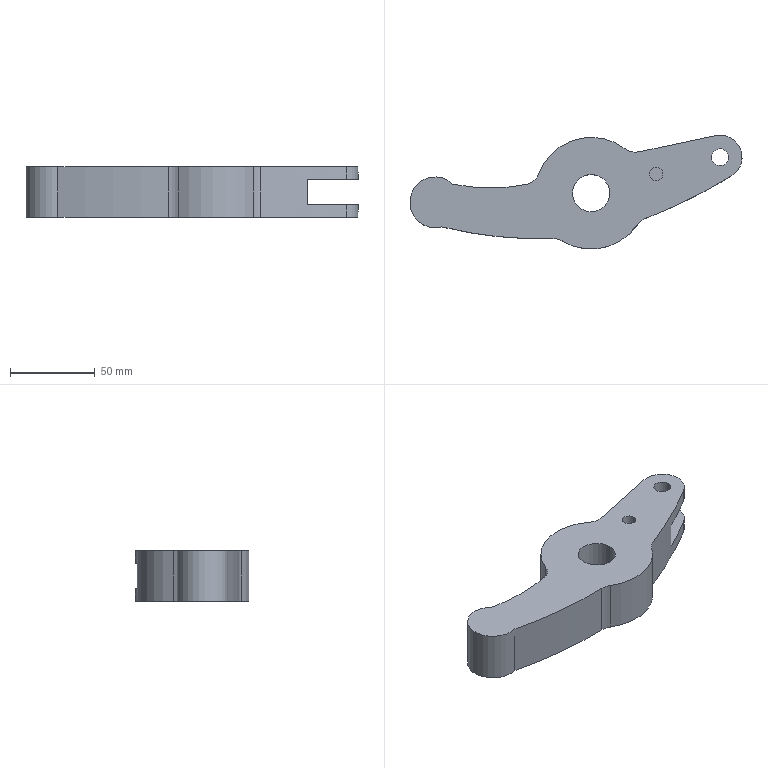Part | SolidWorks | features ICE 15, Cut 1, Extrusion 1, Fillet 1 | 1 solid | 27 faces | box 196.199 x 67.267 x 30 mm | volume 199091 mm3 | cylinder 20 | plane 7 | commonest cylinder face diameters 10 x4 20 x4 8 x2 22 x2 26 x2 66 x2
STEP:
#1=CARTESIAN_POINT('',(135.128,11.377,5.));
#2=VERTEX_POINT('',#1);
#3=CARTESIAN_POINT('',(143.128,11.377,5.));
#4=VERTEX_POINT('',#3);
#5=CARTESIAN_POINT('',(139.128,11.377,5.));
#6=DIRECTION('',(0.,0.,1.));
#7=DIRECTION('',(1.,0.,0.));
#8=AXIS2_PLACEMENT_3D('',#5,#6,#7);
#9=CIRCLE('',#8,4.);
#10=EDGE_CURVE('',#2,#4,#9,.T.);
#11=ORIENTED_EDGE('',*,*,#10,.F.);
#12=CARTESIAN_POINT('',(135.128,11.377,20.));
#13=VERTEX_POINT('',#12);
#14=CARTESIAN_POINT('',(135.128,11.377,5.));
#15=DIRECTION('',(0.,0.,1.));
#16=VECTOR('',#15,1000.);
#17=LINE('',#14,#16);
#18=EDGE_CURVE('',#2,#13,#17,.T.);
#19=ORIENTED_EDGE('',*,*,#18,.T.);
#20=CARTESIAN_POINT('',(143.128,11.377,20.));
#21=VERTEX_POINT('',#20);
#22=CARTESIAN_POINT('',(139.128,11.377,20.));
#23=DIRECTION('',(0.,0.,1.));
#24=DIRECTION('',(1.,0.,0.));
#25=AXIS2_PLACEMENT_3D('',#22,#23,#24);
#26=CIRCLE('',#25,4.);
#27=EDGE_CURVE('',#13,#21,#26,.T.);
#28=ORIENTED_EDGE('',*,*,#27,.T.);
#29=CARTESIAN_POINT('',(143.128,11.377,5.));
#30=DIRECTION('',(0.,0.,1.));
#31=VECTOR('',#30,1000.);
#32=LINE('',#29,#31);
#33=EDGE_CURVE('',#4,#21,#32,.T.);
#34=ORIENTED_EDGE('',*,*,#33,.F.);
#35=EDGE_LOOP('',(#11,#19,#28,#34));
#36=FACE_OUTER_BOUND('',#35,.T.);
#37=CARTESIAN_POINT('',(139.128,11.377,5.));
#38=DIRECTION('',(0.,0.,1.));
#39=DIRECTION('',(1.,0.,0.));
#40=AXIS2_PLACEMENT_3D('',#37,#38,#39);
#41=CYLINDRICAL_SURFACE('',#40,4.);
#42=ADVANCED_FACE('',(#36),#41,.F.);
#43=CARTESIAN_POINT('',(111.78,0.,20.));
#44=VERTEX_POINT('',#43);
#45=CARTESIAN_POINT('',(89.78,0.,20.));
#46=VERTEX_POINT('',#45);
#47=CARTESIAN_POINT('',(100.78,0.,20.));
#48=DIRECTION('',(0.,0.,-1.));
#49=DIRECTION('',(-1.,0.,0.));
#50=AXIS2_PLACEMENT_3D('',#47,#48,#49);
#51=CIRCLE('',#50,11.);
#52=EDGE_CURVE('',#44,#46,#51,.T.);
#53=ORIENTED_EDGE('',*,*,#52,.F.);
#54=CARTESIAN_POINT('',(111.78,0.,-10.));
#55=VERTEX_POINT('',#54);
#56=CARTESIAN_POINT('',(111.78,0.,20.));
#57=DIRECTION('',(0.,0.,-1.));
#58=VECTOR('',#57,1000.);
#59=LINE('',#56,#58);
#60=EDGE_CURVE('',#44,#55,#59,.T.);
#61=ORIENTED_EDGE('',*,*,#60,.T.);
#62=CARTESIAN_POINT('',(89.78,0.,-10.));
#63=VERTEX_POINT('',#62);
#64=CARTESIAN_POINT('',(100.78,0.,-10.));
#65=DIRECTION('',(0.,0.,1.));
#66=DIRECTION('',(1.,0.,0.));
#67=AXIS2_PLACEMENT_3D('',#64,#65,#66);
#68=CIRCLE('',#67,11.);
#69=EDGE_CURVE('',#63,#55,#68,.T.);
#70=ORIENTED_EDGE('',*,*,#69,.F.);
#71=CARTESIAN_POINT('',(89.78,0.,20.));
#72=DIRECTION('',(0.,0.,-1.));
#73=VECTOR('',#72,1000.);
#74=LINE('',#71,#73);
#75=EDGE_CURVE('',#46,#63,#74,.T.);
#76=ORIENTED_EDGE('',*,*,#75,.F.);
#77=EDGE_LOOP('',(#53,#61,#70,#76));
#78=FACE_OUTER_BOUND('',#77,.T.);
#79=CARTESIAN_POINT('',(100.78,0.,20.));
#80=DIRECTION('',(0.,0.,-1.));
#81=DIRECTION('',(-1.,0.,0.));
#82=AXIS2_PLACEMENT_3D('',#79,#80,#81);
#83=CYLINDRICAL_SURFACE('',#82,11.);
#84=ADVANCED_FACE('',(#78),#83,.F.);
#85=CARTESIAN_POINT('',(181.864,21.267,20.));
#86=VERTEX_POINT('',#85);
#87=CARTESIAN_POINT('',(171.864,21.267,20.));
#88=VERTEX_POINT('',#87);
#89=CARTESIAN_POINT('',(176.864,21.267,20.));
#90=DIRECTION('',(0.,0.,-1.));
#91=DIRECTION('',(-1.,0.,0.));
#92=AXIS2_PLACEMENT_3D('',#89,#90,#91);
#93=CIRCLE('',#92,5.);
#94=EDGE_CURVE('',#86,#88,#93,.T.);
#95=ORIENTED_EDGE('',*,*,#94,.F.);
#96=CARTESIAN_POINT('',(181.864,21.267,12.5));
#97=VERTEX_POINT('',#96);
#98=CARTESIAN_POINT('',(181.864,21.267,20.));
#99=DIRECTION('',(0.,0.,-1.));
#100=VECTOR('',#99,1000.);
#101=LINE('',#98,#100);
#102=EDGE_CURVE('',#86,#97,#101,.T.);
#103=ORIENTED_EDGE('',*,*,#102,.T.);
#104=CARTESIAN_POINT('',(171.864,21.267,12.5));
#105=VERTEX_POINT('',#104);
#106=CARTESIAN_POINT('',(176.864,21.267,12.5));
#107=DIRECTION('',(0.,0.,-1.));
#108=DIRECTION('',(1.,0.,0.));
#109=AXIS2_PLACEMENT_3D('',#106,#107,#108);
#110=CIRCLE('',#109,5.);
#111=EDGE_CURVE('',#97,#105,#110,.T.);
#112=ORIENTED_EDGE('',*,*,#111,.T.);
#113=CARTESIAN_POINT('',(171.864,21.267,20.));
#114=DIRECTION('',(0.,0.,-1.));
#115=VECTOR('',#114,1000.);
#116=LINE('',#113,#115);
#117=EDGE_CURVE('',#88,#105,#116,.T.);
#118=ORIENTED_EDGE('',*,*,#117,.F.);
#119=EDGE_LOOP('',(#95,#103,#112,#118));
#120=FACE_OUTER_BOUND('',#119,.T.);
#121=CARTESIAN_POINT('',(176.864,21.267,20.));
#122=DIRECTION('',(0.,0.,-1.));
#123=DIRECTION('',(-1.,0.,0.));
#124=AXIS2_PLACEMENT_3D('',#121,#122,#123);
#125=CYLINDRICAL_SURFACE('',#124,5.);
#126=ADVANCED_FACE('',(#120),#125,.F.);
#127=CARTESIAN_POINT('',(181.864,21.267,-2.5));
#128=VERTEX_POINT('',#127);
#129=CARTESIAN_POINT('',(171.864,21.267,-2.5));
#130=VERTEX_POINT('',#129);
#131=CARTESIAN_POINT('',(176.864,21.267,-2.5));
#132=DIRECTION('',(0.,0.,-1.));
#133=DIRECTION('',(1.,0.,0.));
#134=AXIS2_PLACEMENT_3D('',#131,#132,#133);
#135=CIRCLE('',#134,5.);
#136=EDGE_CURVE('',#128,#130,#135,.T.);
#137=ORIENTED_EDGE('',*,*,#136,.F.);
#138=CARTESIAN_POINT('',(181.864,21.267,-10.));
#139=VERTEX_POINT('',#138);
#140=CARTESIAN_POINT('',(181.864,21.267,20.));
#141=DIRECTION('',(0.,0.,-1.));
#142=VECTOR('',#141,1000.);
#143=LINE('',#140,#142);
#144=EDGE_CURVE('',#128,#139,#143,.T.);
#145=ORIENTED_EDGE('',*,*,#144,.T.);
#146=CARTESIAN_POINT('',(171.864,21.267,-10.));
#147=VERTEX_POINT('',#146);
#148=CARTESIAN_POINT('',(176.864,21.267,-10.));
#149=DIRECTION('',(0.,0.,1.));
#150=DIRECTION('',(1.,0.,0.));
#151=AXIS2_PLACEMENT_3D('',#148,#149,#150);
#152=CIRCLE('',#151,5.);
#153=EDGE_CURVE('',#147,#139,#152,.T.);
#154=ORIENTED_EDGE('',*,*,#153,.F.);
#155=CARTESIAN_POINT('',(171.864,21.267,20.));
#156=DIRECTION('',(0.,0.,-1.));
#157=VECTOR('',#156,1000.);
#158=LINE('',#155,#157);
#159=EDGE_CURVE('',#130,#147,#158,.T.);
#160=ORIENTED_EDGE('',*,*,#159,.F.);
#161=EDGE_LOOP('',(#137,#145,#154,#160));
#162=FACE_OUTER_BOUND('',#161,.T.);
#163=CARTESIAN_POINT('',(176.864,21.267,20.));
#164=DIRECTION('',(0.,0.,-1.));
#165=DIRECTION('',(-1.,0.,0.));
#166=AXIS2_PLACEMENT_3D('',#163,#164,#165);
#167=CYLINDRICAL_SURFACE('',#166,5.);
#168=ADVANCED_FACE('',(#162),#167,.F.);
#169=CARTESIAN_POINT('',(183.231,9.933,20.));
#170=VERTEX_POINT('',#169);
#171=CARTESIAN_POINT('',(132.488,-15.137,20.));
#172=VERTEX_POINT('',#171);
#173=CARTESIAN_POINT('',(6.853,303.042,20.));
#174=DIRECTION('',(0.,0.,-1.));
#175=DIRECTION('',(1.,0.,0.));
#176=AXIS2_PLACEMENT_3D('',#173,#174,#175);
#177=CIRCLE('',#176,342.085);
#178=EDGE_CURVE('',#170,#172,#177,.T.);
#179=ORIENTED_EDGE('',*,*,#178,.T.);
#180=CARTESIAN_POINT('',(132.488,-15.137,-10.));
#181=VERTEX_POINT('',#180);
#182=CARTESIAN_POINT('',(132.488,-15.137,202.081));
#183=DIRECTION('',(0.,0.,-1.));
#184=VECTOR('',#183,1000.);
#185=LINE('',#182,#184);
#186=EDGE_CURVE('',#172,#181,#185,.T.);
#187=ORIENTED_EDGE('',*,*,#186,.T.);
#188=CARTESIAN_POINT('',(183.231,9.933,-10.));
#189=VERTEX_POINT('',#188);
#190=CARTESIAN_POINT('',(6.853,303.042,-10.));
#191=DIRECTION('',(0.,0.,-1.));
#192=DIRECTION('',(-1.,0.,0.));
#193=AXIS2_PLACEMENT_3D('',#190,#191,#192);
#194=CIRCLE('',#193,342.085);
#195=EDGE_CURVE('',#189,#181,#194,.T.);
#196=ORIENTED_EDGE('',*,*,#195,.F.);
#197=CARTESIAN_POINT('',(183.231,9.933,-2.5));
#198=VERTEX_POINT('',#197);
#199=CARTESIAN_POINT('',(183.231,9.933,5.));
#200=DIRECTION('',(0.,0.,1.));
#201=VECTOR('',#200,1000.);
#202=LINE('',#199,#201);
#203=EDGE_CURVE('',#189,#198,#202,.T.);
#204=ORIENTED_EDGE('',*,*,#203,.T.);
#205=CARTESIAN_POINT('',(159.864,-2.915,-2.5));
#206=VERTEX_POINT('',#205);
#207=CARTESIAN_POINT('',(6.853,303.042,-2.5));
#208=DIRECTION('',(0.,0.,-1.));
#209=DIRECTION('',(1.,0.,0.));
#210=AXIS2_PLACEMENT_3D('',#207,#208,#209);
#211=CIRCLE('',#210,342.085);
#212=EDGE_CURVE('',#198,#206,#211,.T.);
#213=ORIENTED_EDGE('',*,*,#212,.T.);
#214=CARTESIAN_POINT('',(159.864,-2.915,12.5));
#215=VERTEX_POINT('',#214);
#216=CARTESIAN_POINT('',(159.864,-2.915,202.081));
#217=DIRECTION('',(0.,0.,1.));
#218=VECTOR('',#217,1000.);
#219=LINE('',#216,#218);
#220=EDGE_CURVE('',#206,#215,#219,.T.);
#221=ORIENTED_EDGE('',*,*,#220,.T.);
#222=CARTESIAN_POINT('',(183.231,9.933,12.5));
#223=VERTEX_POINT('',#222);
#224=CARTESIAN_POINT('',(6.853,303.042,12.5));
#225=DIRECTION('',(0.,0.,1.));
#226=DIRECTION('',(-1.,0.,0.));
#227=AXIS2_PLACEMENT_3D('',#224,#225,#226);
#228=CIRCLE('',#227,342.085);
#229=EDGE_CURVE('',#215,#223,#228,.T.);
#230=ORIENTED_EDGE('',*,*,#229,.T.);
#231=CARTESIAN_POINT('',(183.231,9.933,5.));
#232=DIRECTION('',(0.,0.,-1.));
#233=VECTOR('',#232,1000.);
#234=LINE('',#231,#233);
#235=EDGE_CURVE('',#170,#223,#234,.T.);
#236=ORIENTED_EDGE('',*,*,#235,.F.);
#237=EDGE_LOOP('',(#179,#187,#196,#204,#213,#221,#230,#236));
#238=FACE_OUTER_BOUND('',#237,.T.);
#239=CARTESIAN_POINT('',(6.853,303.042,202.081));
#240=DIRECTION('',(0.,0.,-1.));
#241=DIRECTION('',(-1.,0.,0.));
#242=AXIS2_PLACEMENT_3D('',#239,#240,#241);
#243=CYLINDRICAL_SURFACE('',#242,342.085);
#244=ADVANCED_FACE('',(#238),#243,.T.);
#245=CARTESIAN_POINT('',(78.197,-26.796,20.));
#246=VERTEX_POINT('',#245);
#247=CARTESIAN_POINT('',(12.608,-19.89,20.));
#248=VERTEX_POINT('',#247);
#249=CARTESIAN_POINT('',(70.404,214.131,20.));
#250=DIRECTION('',(0.,0.,-1.));
#251=DIRECTION('',(1.,0.,0.));
#252=AXIS2_PLACEMENT_3D('',#249,#250,#251);
#253=CIRCLE('',#252,241.052);
#254=EDGE_CURVE('',#246,#248,#253,.T.);
#255=ORIENTED_EDGE('',*,*,#254,.T.);
#256=CARTESIAN_POINT('',(12.608,-19.89,-10.));
#257=VERTEX_POINT('',#256);
#258=CARTESIAN_POINT('',(12.608,-19.89,-102.078));
#259=DIRECTION('',(0.,0.,1.));
#260=VECTOR('',#259,1000.);
#261=LINE('',#258,#260);
#262=EDGE_CURVE('',#257,#248,#261,.T.);
#263=ORIENTED_EDGE('',*,*,#262,.F.);
#264=CARTESIAN_POINT('',(78.197,-26.796,-10.));
#265=VERTEX_POINT('',#264);
#266=CARTESIAN_POINT('',(70.404,214.131,-10.));
#267=DIRECTION('',(0.,0.,-1.));
#268=DIRECTION('',(1.,0.,0.));
#269=AXIS2_PLACEMENT_3D('',#266,#267,#268);
#270=CIRCLE('',#269,241.052);
#271=EDGE_CURVE('',#265,#257,#270,.T.);
#272=ORIENTED_EDGE('',*,*,#271,.F.);
#273=CARTESIAN_POINT('',(78.197,-26.796,202.081));
#274=DIRECTION('',(0.,0.,1.));
#275=VECTOR('',#274,1000.);
#276=LINE('',#273,#275);
#277=EDGE_CURVE('',#265,#246,#276,.T.);
#278=ORIENTED_EDGE('',*,*,#277,.T.);
#279=EDGE_LOOP('',(#255,#263,#272,#278));
#280=FACE_OUTER_BOUND('',#279,.T.);
#281=CARTESIAN_POINT('',(70.404,214.131,202.081));
#282=DIRECTION('',(0.,0.,-1.));
#283=DIRECTION('',(-1.,0.,0.));
#284=AXIS2_PLACEMENT_3D('',#281,#282,#283);
#285=CYLINDRICAL_SURFACE('',#284,241.052);
#286=ADVANCED_FACE('',(#280),#285,.T.);
#287=CARTESIAN_POINT('',(69.859,11.528,20.));
#288=VERTEX_POINT('',#287);
#289=CARTESIAN_POINT('',(62.463,5.218,20.));
#290=VERTEX_POINT('',#289);
#291=CARTESIAN_POINT('',(60.489,15.021,20.));
#292=DIRECTION('',(0.,0.,-1.));
#293=DIRECTION('',(1.,0.,0.));
#294=AXIS2_PLACEMENT_3D('',#291,#292,#293);
#295=CIRCLE('',#294,10.);
#296=EDGE_CURVE('',#288,#290,#295,.T.);
#297=ORIENTED_EDGE('',*,*,#296,.T.);
#298=CARTESIAN_POINT('',(19.079,5.378,20.));
#299=VERTEX_POINT('',#298);
#300=CARTESIAN_POINT('',(41.161,110.985,20.));
#301=DIRECTION('',(0.,0.,-1.));
#302=DIRECTION('',(1.,0.,0.));
#303=AXIS2_PLACEMENT_3D('',#300,#301,#302);
#304=CIRCLE('',#303,107.891);
#305=EDGE_CURVE('',#290,#299,#304,.T.);
#306=ORIENTED_EDGE('',*,*,#305,.T.);
#307=CARTESIAN_POINT('',(8.665,-5.418,20.));
#308=DIRECTION('',(0.,0.,1.));
#309=DIRECTION('',(1.,0.,0.));
#310=AXIS2_PLACEMENT_3D('',#307,#308,#309);
#311=CIRCLE('',#310,15.);
#312=EDGE_CURVE('',#299,#248,#311,.T.);
#313=ORIENTED_EDGE('',*,*,#312,.T.);
#314=ORIENTED_EDGE('',*,*,#254,.F.);
#315=CARTESIAN_POINT('',(83.697,-28.234,20.));
#316=VERTEX_POINT('',#315);
#317=CARTESIAN_POINT('',(78.521,-36.79,20.));
#318=DIRECTION('',(0.,0.,-1.));
#319=DIRECTION('',(1.,0.,0.));
#320=AXIS2_PLACEMENT_3D('',#317,#318,#319);
#321=CIRCLE('',#320,10.);
#322=EDGE_CURVE('',#246,#316,#321,.T.);
#323=ORIENTED_EDGE('',*,*,#322,.T.);
#324=CARTESIAN_POINT('',(127.932,-18.755,20.));
#325=VERTEX_POINT('',#324);
#326=CARTESIAN_POINT('',(100.78,0.,20.));
#327=DIRECTION('',(0.,0.,1.));
#328=DIRECTION('',(1.,0.,0.));
#329=AXIS2_PLACEMENT_3D('',#326,#327,#328);
#330=CIRCLE('',#329,33.);
#331=EDGE_CURVE('',#316,#325,#330,.T.);
#332=ORIENTED_EDGE('',*,*,#331,.T.);
#333=CARTESIAN_POINT('',(136.16,-24.439,20.));
#334=DIRECTION('',(0.,0.,-1.));
#335=DIRECTION('',(1.,0.,0.));
#336=AXIS2_PLACEMENT_3D('',#333,#334,#335);
#337=CIRCLE('',#336,10.);
#338=EDGE_CURVE('',#325,#172,#337,.T.);
#339=ORIENTED_EDGE('',*,*,#338,.T.);
#340=ORIENTED_EDGE('',*,*,#178,.F.);
#341=CARTESIAN_POINT('',(183.921,10.349,20.));
#342=VERTEX_POINT('',#341);
#343=CARTESIAN_POINT('',(183.231,9.933,20.));
#344=CARTESIAN_POINT('',(183.461,10.072,20.));
#345=CARTESIAN_POINT('',(183.691,10.211,20.));
#346=CARTESIAN_POINT('',(183.921,10.349,20.));
#347=B_SPLINE_CURVE_WITH_KNOTS('',3,(#343,#344,#345,#346),.UNSPECIFIED.,.F.,.F.,(4,4),(0.,1.),.UNSPECIFIED.);
#348=EDGE_CURVE('',#170,#342,#347,.T.);
#349=ORIENTED_EDGE('',*,*,#348,.T.);
#350=CARTESIAN_POINT('',(174.169,33.984,20.));
#351=VERTEX_POINT('',#350);
#352=CARTESIAN_POINT('',(176.864,21.267,20.));
#353=DIRECTION('',(0.,0.,1.));
#354=DIRECTION('',(1.,0.,0.));
#355=AXIS2_PLACEMENT_3D('',#352,#353,#354);
#356=CIRCLE('',#355,13.);
#357=EDGE_CURVE('',#342,#351,#356,.T.);
#358=ORIENTED_EDGE('',*,*,#357,.T.);
#359=CARTESIAN_POINT('',(128.939,24.401,20.));
#360=VERTEX_POINT('',#359);
#361=CARTESIAN_POINT('',(174.169,33.984,20.));
#362=DIRECTION('',(-0.9783,-0.2073,0.));
#363=VECTOR('',#362,1000.);
#364=LINE('',#361,#363);
#365=EDGE_CURVE('',#351,#360,#364,.T.);
#366=ORIENTED_EDGE('',*,*,#365,.T.);
#367=CARTESIAN_POINT('',(120.8,26.234,20.));
#368=VERTEX_POINT('',#367);
#369=CARTESIAN_POINT('',(126.866,34.184,20.));
#370=DIRECTION('',(0.,0.,-1.));
#371=DIRECTION('',(1.,0.,0.));
#372=AXIS2_PLACEMENT_3D('',#369,#370,#371);
#373=CIRCLE('',#372,10.);
#374=EDGE_CURVE('',#360,#368,#373,.T.);
#375=ORIENTED_EDGE('',*,*,#374,.T.);
#376=CARTESIAN_POINT('',(100.78,0.,20.));
#377=DIRECTION('',(0.,0.,1.));
#378=DIRECTION('',(1.,0.,0.));
#379=AXIS2_PLACEMENT_3D('',#376,#377,#378);
#380=CIRCLE('',#379,33.);
#381=EDGE_CURVE('',#368,#288,#380,.T.);
#382=ORIENTED_EDGE('',*,*,#381,.T.);
#383=EDGE_LOOP('',(#297,#306,#313,#314,#323,#332,#339,#340,#349,#358,#366,#375,#382));
#384=FACE_OUTER_BOUND('',#383,.T.);
#385=CARTESIAN_POINT('',(139.128,11.377,20.));
#386=DIRECTION('',(0.,0.,1.));
#387=DIRECTION('',(1.,0.,0.));
#388=AXIS2_PLACEMENT_3D('',#385,#386,#387);
#389=CIRCLE('',#388,4.);
#390=EDGE_CURVE('',#21,#13,#389,.T.);
#391=ORIENTED_EDGE('',*,*,#390,.F.);
#392=ORIENTED_EDGE('',*,*,#27,.F.);
#393=EDGE_LOOP('',(#391,#392));
#394=FACE_BOUND('',#393,.T.);
#395=CARTESIAN_POINT('',(176.864,21.267,20.));
#396=DIRECTION('',(0.,0.,-1.));
#397=DIRECTION('',(-1.,0.,0.));
#398=AXIS2_PLACEMENT_3D('',#395,#396,#397);
#399=CIRCLE('',#398,5.);
#400=EDGE_CURVE('',#88,#86,#399,.T.);
#401=ORIENTED_EDGE('',*,*,#400,.T.);
#402=ORIENTED_EDGE('',*,*,#94,.T.);
#403=EDGE_LOOP('',(#401,#402));
#404=FACE_BOUND('',#403,.T.);
#405=CARTESIAN_POINT('',(100.78,0.,20.));
#406=DIRECTION('',(0.,0.,-1.));
#407=DIRECTION('',(-1.,0.,0.));
#408=AXIS2_PLACEMENT_3D('',#405,#406,#407);
#409=CIRCLE('',#408,11.);
#410=EDGE_CURVE('',#46,#44,#409,.T.);
#411=ORIENTED_EDGE('',*,*,#410,.T.);
#412=ORIENTED_EDGE('',*,*,#52,.T.);
#413=EDGE_LOOP('',(#411,#412));
#414=FACE_BOUND('',#413,.T.);
#415=CARTESIAN_POINT('',(8.665,-5.418,20.));
#416=DIRECTION('',(0.,0.,1.));
#417=DIRECTION('',(1.,0.,0.));
#418=AXIS2_PLACEMENT_3D('',#415,#416,#417);
#419=PLANE('',#418);
#420=ADVANCED_FACE('',(#384,#394,#404,#414),#419,.T.);
#421=ORIENTED_EDGE('',*,*,#271,.T.);
#422=CARTESIAN_POINT('',(19.079,5.378,-10.));
#423=VERTEX_POINT('',#422);
#424=CARTESIAN_POINT('',(8.665,-5.418,-10.));
#425=DIRECTION('',(0.,0.,1.));
#426=DIRECTION('',(-1.,0.,0.));
#427=AXIS2_PLACEMENT_3D('',#424,#425,#426);
#428=CIRCLE('',#427,15.);
#429=EDGE_CURVE('',#423,#257,#428,.T.);
#430=ORIENTED_EDGE('',*,*,#429,.F.);
#431=CARTESIAN_POINT('',(62.463,5.218,-10.));
#432=VERTEX_POINT('',#431);
#433=CARTESIAN_POINT('',(41.161,110.985,-10.));
#434=DIRECTION('',(0.,0.,-1.));
#435=DIRECTION('',(-1.,0.,0.));
#436=AXIS2_PLACEMENT_3D('',#433,#434,#435);
#437=CIRCLE('',#436,107.891);
#438=EDGE_CURVE('',#432,#423,#437,.T.);
#439=ORIENTED_EDGE('',*,*,#438,.F.);
#440=CARTESIAN_POINT('',(69.859,11.528,-10.));
#441=VERTEX_POINT('',#440);
#442=CARTESIAN_POINT('',(60.489,15.021,-10.));
#443=DIRECTION('',(0.,0.,1.));
#444=DIRECTION('',(-1.,0.,0.));
#445=AXIS2_PLACEMENT_3D('',#442,#443,#444);
#446=CIRCLE('',#445,10.);
#447=EDGE_CURVE('',#432,#441,#446,.T.);
#448=ORIENTED_EDGE('',*,*,#447,.T.);
#449=CARTESIAN_POINT('',(120.8,26.234,-10.));
#450=VERTEX_POINT('',#449);
#451=CARTESIAN_POINT('',(100.78,0.,-10.));
#452=DIRECTION('',(0.,0.,1.));
#453=DIRECTION('',(-1.,0.,0.));
#454=AXIS2_PLACEMENT_3D('',#451,#452,#453);
#455=CIRCLE('',#454,33.);
#456=EDGE_CURVE('',#450,#441,#455,.T.);
#457=ORIENTED_EDGE('',*,*,#456,.F.);
#458=CARTESIAN_POINT('',(128.939,24.401,-10.));
#459=VERTEX_POINT('',#458);
#460=CARTESIAN_POINT('',(126.866,34.184,-10.));
#461=DIRECTION('',(0.,0.,1.));
#462=DIRECTION('',(-1.,0.,0.));
#463=AXIS2_PLACEMENT_3D('',#460,#461,#462);
#464=CIRCLE('',#463,10.);
#465=EDGE_CURVE('',#450,#459,#464,.T.);
#466=ORIENTED_EDGE('',*,*,#465,.T.);
#467=CARTESIAN_POINT('',(174.169,33.984,-10.));
#468=VERTEX_POINT('',#467);
#469=CARTESIAN_POINT('',(97.09,17.652,-10.));
#470=DIRECTION('',(0.9783,0.2073,0.));
#471=VECTOR('',#470,1000.);
#472=LINE('',#469,#471);
#473=EDGE_CURVE('',#459,#468,#472,.T.);
#474=ORIENTED_EDGE('',*,*,#473,.T.);
#475=CARTESIAN_POINT('',(183.921,10.349,-10.));
#476=VERTEX_POINT('',#475);
#477=CARTESIAN_POINT('',(176.864,21.267,-10.));
#478=DIRECTION('',(0.,0.,-1.));
#479=DIRECTION('',(-1.,0.,0.));
#480=AXIS2_PLACEMENT_3D('',#477,#478,#479);
#481=CIRCLE('',#480,13.);
#482=EDGE_CURVE('',#468,#476,#481,.T.);
#483=ORIENTED_EDGE('',*,*,#482,.T.);
#484=CARTESIAN_POINT('',(183.921,10.349,-10.));
#485=CARTESIAN_POINT('',(183.691,10.211,-10.));
#486=CARTESIAN_POINT('',(183.461,10.072,-10.));
#487=CARTESIAN_POINT('',(183.231,9.933,-10.));
#488=B_SPLINE_CURVE_WITH_KNOTS('',3,(#484,#485,#486,#487),.UNSPECIFIED.,.F.,.F.,(4,4),(0.,1.),.UNSPECIFIED.);
#489=EDGE_CURVE('',#476,#189,#488,.T.);
#490=ORIENTED_EDGE('',*,*,#489,.T.);
#491=ORIENTED_EDGE('',*,*,#195,.T.);
#492=CARTESIAN_POINT('',(127.932,-18.755,-10.));
#493=VERTEX_POINT('',#492);
#494=CARTESIAN_POINT('',(136.16,-24.439,-10.));
#495=DIRECTION('',(0.,0.,1.));
#496=DIRECTION('',(-1.,0.,0.));
#497=AXIS2_PLACEMENT_3D('',#494,#495,#496);
#498=CIRCLE('',#497,10.);
#499=EDGE_CURVE('',#181,#493,#498,.T.);
#500=ORIENTED_EDGE('',*,*,#499,.T.);
#501=CARTESIAN_POINT('',(83.697,-28.234,-10.));
#502=VERTEX_POINT('',#501);
#503=CARTESIAN_POINT('',(100.78,0.,-10.));
#504=DIRECTION('',(0.,0.,1.));
#505=DIRECTION('',(-1.,0.,0.));
#506=AXIS2_PLACEMENT_3D('',#503,#504,#505);
#507=CIRCLE('',#506,33.);
#508=EDGE_CURVE('',#502,#493,#507,.T.);
#509=ORIENTED_EDGE('',*,*,#508,.F.);
#510=CARTESIAN_POINT('',(78.521,-36.79,-10.));
#511=DIRECTION('',(0.,0.,1.));
#512=DIRECTION('',(-1.,0.,0.));
#513=AXIS2_PLACEMENT_3D('',#510,#511,#512);
#514=CIRCLE('',#513,10.);
#515=EDGE_CURVE('',#502,#265,#514,.T.);
#516=ORIENTED_EDGE('',*,*,#515,.T.);
#517=EDGE_LOOP('',(#421,#430,#439,#448,#457,#466,#474,#483,#490,#491,#500,#509,#516));
#518=FACE_OUTER_BOUND('',#517,.T.);
#519=ORIENTED_EDGE('',*,*,#69,.T.);
#520=CARTESIAN_POINT('',(100.78,0.,-10.));
#521=DIRECTION('',(0.,0.,1.));
#522=DIRECTION('',(1.,0.,0.));
#523=AXIS2_PLACEMENT_3D('',#520,#521,#522);
#524=CIRCLE('',#523,11.);
#525=EDGE_CURVE('',#55,#63,#524,.T.);
#526=ORIENTED_EDGE('',*,*,#525,.T.);
#527=EDGE_LOOP('',(#519,#526));
#528=FACE_BOUND('',#527,.T.);
#529=ORIENTED_EDGE('',*,*,#153,.T.);
#530=CARTESIAN_POINT('',(176.864,21.267,-10.));
#531=DIRECTION('',(0.,0.,1.));
#532=DIRECTION('',(1.,0.,0.));
#533=AXIS2_PLACEMENT_3D('',#530,#531,#532);
#534=CIRCLE('',#533,5.);
#535=EDGE_CURVE('',#139,#147,#534,.T.);
#536=ORIENTED_EDGE('',*,*,#535,.T.);
#537=EDGE_LOOP('',(#529,#536));
#538=FACE_BOUND('',#537,.T.);
#539=CARTESIAN_POINT('',(100.506,-0.02055,-10.));
#540=DIRECTION('',(0.,0.,-1.));
#541=DIRECTION('',(-1.,0.,0.));
#542=AXIS2_PLACEMENT_3D('',#539,#540,#541);
#543=PLANE('',#542);
#544=ADVANCED_FACE('',(#518,#528,#538),#543,.T.);
#545=ORIENTED_EDGE('',*,*,#229,.F.);
#546=CARTESIAN_POINT('',(159.864,30.953,12.5));
#547=VERTEX_POINT('',#546);
#548=CARTESIAN_POINT('',(159.864,-3.573,12.5));
#549=DIRECTION('',(0.,1.,0.));
#550=VECTOR('',#549,1000.);
#551=LINE('',#548,#550);
#552=EDGE_CURVE('',#215,#547,#551,.T.);
#553=ORIENTED_EDGE('',*,*,#552,.T.);
#554=CARTESIAN_POINT('',(174.169,33.984,12.5));
#555=VERTEX_POINT('',#554);
#556=CARTESIAN_POINT('',(174.169,33.984,12.5));
#557=DIRECTION('',(-0.9783,-0.2073,0.));
#558=VECTOR('',#557,1000.);
#559=LINE('',#556,#558);
#560=EDGE_CURVE('',#555,#547,#559,.T.);
#561=ORIENTED_EDGE('',*,*,#560,.F.);
#562=CARTESIAN_POINT('',(183.921,10.349,12.5));
#563=VERTEX_POINT('',#562);
#564=CARTESIAN_POINT('',(176.864,21.267,12.5));
#565=DIRECTION('',(0.,0.,1.));
#566=DIRECTION('',(1.,0.,0.));
#567=AXIS2_PLACEMENT_3D('',#564,#565,#566);
#568=CIRCLE('',#567,13.);
#569=EDGE_CURVE('',#563,#555,#568,.T.);
#570=ORIENTED_EDGE('',*,*,#569,.F.);
#571=CARTESIAN_POINT('',(183.231,9.933,12.5));
#572=CARTESIAN_POINT('',(183.466,10.065,12.5));
#573=CARTESIAN_POINT('',(183.696,10.204,12.5));
#574=CARTESIAN_POINT('',(183.921,10.349,12.5));
#575=B_SPLINE_CURVE_WITH_KNOTS('',3,(#571,#572,#573,#574),.UNSPECIFIED.,.F.,.F.,(4,4),(0.,1.),.UNSPECIFIED.);
#576=EDGE_CURVE('',#223,#563,#575,.T.);
#577=ORIENTED_EDGE('',*,*,#576,.F.);
#578=EDGE_LOOP('',(#545,#553,#561,#570,#577));
#579=FACE_OUTER_BOUND('',#578,.T.);
#580=CARTESIAN_POINT('',(176.864,21.267,12.5));
#581=DIRECTION('',(0.,0.,-1.));
#582=DIRECTION('',(1.,0.,0.));
#583=AXIS2_PLACEMENT_3D('',#580,#581,#582);
#584=CIRCLE('',#583,5.);
#585=EDGE_CURVE('',#105,#97,#584,.T.);
#586=ORIENTED_EDGE('',*,*,#585,.F.);
#587=ORIENTED_EDGE('',*,*,#111,.F.);
#588=EDGE_LOOP('',(#586,#587));
#589=FACE_BOUND('',#588,.T.);
#590=CARTESIAN_POINT('',(0.,0.,12.5));
#591=DIRECTION('',(0.,0.,1.));
#592=DIRECTION('',(1.,0.,0.));
#593=AXIS2_PLACEMENT_3D('',#590,#591,#592);
#594=PLANE('',#593);
#595=ADVANCED_FACE('',(#579,#589),#594,.F.);
#596=CARTESIAN_POINT('',(159.864,30.953,-2.5));
#597=VERTEX_POINT('',#596);
#598=CARTESIAN_POINT('',(159.864,-3.573,-2.5));
#599=DIRECTION('',(0.,1.,0.));
#600=VECTOR('',#599,1000.);
#601=LINE('',#598,#600);
#602=EDGE_CURVE('',#206,#597,#601,.T.);
#603=ORIENTED_EDGE('',*,*,#602,.F.);
#604=ORIENTED_EDGE('',*,*,#212,.F.);
#605=CARTESIAN_POINT('',(183.921,10.349,-2.5));
#606=VERTEX_POINT('',#605);
#607=CARTESIAN_POINT('',(183.921,10.349,-2.5));
#608=CARTESIAN_POINT('',(183.696,10.204,-2.5));
#609=CARTESIAN_POINT('',(183.466,10.065,-2.5));
#610=CARTESIAN_POINT('',(183.231,9.933,-2.5));
#611=B_SPLINE_CURVE_WITH_KNOTS('',3,(#607,#608,#609,#610),.UNSPECIFIED.,.F.,.F.,(4,4),(0.,1.),.UNSPECIFIED.);
#612=EDGE_CURVE('',#606,#198,#611,.T.);
#613=ORIENTED_EDGE('',*,*,#612,.F.);
#614=CARTESIAN_POINT('',(174.169,33.984,-2.5));
#615=VERTEX_POINT('',#614);
#616=CARTESIAN_POINT('',(176.864,21.267,-2.5));
#617=DIRECTION('',(0.,0.,-1.));
#618=DIRECTION('',(1.,0.,0.));
#619=AXIS2_PLACEMENT_3D('',#616,#617,#618);
#620=CIRCLE('',#619,13.);
#621=EDGE_CURVE('',#615,#606,#620,.T.);
#622=ORIENTED_EDGE('',*,*,#621,.F.);
#623=CARTESIAN_POINT('',(174.169,33.984,-2.5));
#624=DIRECTION('',(-0.9783,-0.2073,0.));
#625=VECTOR('',#624,1000.);
#626=LINE('',#623,#625);
#627=EDGE_CURVE('',#615,#597,#626,.T.);
#628=ORIENTED_EDGE('',*,*,#627,.T.);
#629=EDGE_LOOP('',(#603,#604,#613,#622,#628));
#630=FACE_OUTER_BOUND('',#629,.T.);
#631=CARTESIAN_POINT('',(176.864,21.267,-2.5));
#632=DIRECTION('',(0.,0.,-1.));
#633=DIRECTION('',(1.,0.,0.));
#634=AXIS2_PLACEMENT_3D('',#631,#632,#633);
#635=CIRCLE('',#634,5.);
#636=EDGE_CURVE('',#130,#128,#635,.T.);
#637=ORIENTED_EDGE('',*,*,#636,.T.);
#638=ORIENTED_EDGE('',*,*,#136,.T.);
#639=EDGE_LOOP('',(#637,#638));
#640=FACE_BOUND('',#639,.T.);
#641=CARTESIAN_POINT('',(0.,0.,-2.5));
#642=DIRECTION('',(0.,0.,1.));
#643=DIRECTION('',(1.,0.,0.));
#644=AXIS2_PLACEMENT_3D('',#641,#642,#643);
#645=PLANE('',#644);
#646=ADVANCED_FACE('',(#630,#640),#645,.T.);
#647=ORIENTED_EDGE('',*,*,#438,.T.);
#648=CARTESIAN_POINT('',(19.079,5.378,-102.078));
#649=DIRECTION('',(0.,0.,1.));
#650=VECTOR('',#649,1000.);
#651=LINE('',#648,#650);
#652=EDGE_CURVE('',#423,#299,#651,.T.);
#653=ORIENTED_EDGE('',*,*,#652,.T.);
#654=ORIENTED_EDGE('',*,*,#305,.F.);
#655=CARTESIAN_POINT('',(62.463,5.218,20.));
#656=DIRECTION('',(0.,0.,-1.));
#657=VECTOR('',#656,1000.);
#658=LINE('',#655,#657);
#659=EDGE_CURVE('',#290,#432,#658,.T.);
#660=ORIENTED_EDGE('',*,*,#659,.T.);
#661=EDGE_LOOP('',(#647,#653,#654,#660));
#662=FACE_OUTER_BOUND('',#661,.T.);
#663=CARTESIAN_POINT('',(41.161,110.985,20.));
#664=DIRECTION('',(0.,0.,-1.));
#665=DIRECTION('',(-1.,0.,0.));
#666=AXIS2_PLACEMENT_3D('',#663,#664,#665);
#667=CYLINDRICAL_SURFACE('',#666,107.891);
#668=ADVANCED_FACE('',(#662),#667,.F.);
#669=ORIENTED_EDGE('',*,*,#144,.F.);
#670=ORIENTED_EDGE('',*,*,#636,.F.);
#671=ORIENTED_EDGE('',*,*,#159,.T.);
#672=ORIENTED_EDGE('',*,*,#535,.F.);
#673=EDGE_LOOP('',(#669,#670,#671,#672));
#674=FACE_OUTER_BOUND('',#673,.T.);
#675=CARTESIAN_POINT('',(176.864,21.267,20.));
#676=DIRECTION('',(0.,0.,-1.));
#677=DIRECTION('',(-1.,0.,0.));
#678=AXIS2_PLACEMENT_3D('',#675,#676,#677);
#679=CYLINDRICAL_SURFACE('',#678,5.);
#680=ADVANCED_FACE('',(#674),#679,.F.);
#681=ORIENTED_EDGE('',*,*,#489,.F.);
#682=ORIENTED_EDGE('',*,*,#482,.F.);
#683=CARTESIAN_POINT('',(174.169,33.984,10.));
#684=DIRECTION('',(0.,0.,-1.));
#685=VECTOR('',#684,1000.);
#686=LINE('',#683,#685);
#687=EDGE_CURVE('',#615,#468,#686,.T.);
#688=ORIENTED_EDGE('',*,*,#687,.F.);
#689=ORIENTED_EDGE('',*,*,#621,.T.);
#690=ORIENTED_EDGE('',*,*,#612,.T.);
#691=ORIENTED_EDGE('',*,*,#203,.F.);
#692=EDGE_LOOP('',(#681,#682,#688,#689,#690,#691));
#693=FACE_OUTER_BOUND('',#692,.T.);
#694=CARTESIAN_POINT('',(176.864,21.267,10.));
#695=DIRECTION('',(0.,0.,-1.));
#696=DIRECTION('',(-1.,0.,0.));
#697=AXIS2_PLACEMENT_3D('',#694,#695,#696);
#698=CYLINDRICAL_SURFACE('',#697,13.);
#699=ADVANCED_FACE('',(#693),#698,.T.);
#700=ORIENTED_EDGE('',*,*,#473,.F.);
#701=CARTESIAN_POINT('',(128.939,24.401,20.));
#702=DIRECTION('',(0.,0.,1.));
#703=VECTOR('',#702,1000.);
#704=LINE('',#701,#703);
#705=EDGE_CURVE('',#459,#360,#704,.T.);
#706=ORIENTED_EDGE('',*,*,#705,.T.);
#707=ORIENTED_EDGE('',*,*,#365,.F.);
#708=CARTESIAN_POINT('',(174.169,33.984,20.));
#709=DIRECTION('',(0.,0.,-1.));
#710=VECTOR('',#709,1000.);
#711=LINE('',#708,#710);
#712=EDGE_CURVE('',#351,#555,#711,.T.);
#713=ORIENTED_EDGE('',*,*,#712,.T.);
#714=ORIENTED_EDGE('',*,*,#560,.T.);
#715=CARTESIAN_POINT('',(159.864,30.953,20.));
#716=DIRECTION('',(0.,0.,-1.));
#717=VECTOR('',#716,1000.);
#718=LINE('',#715,#717);
#719=EDGE_CURVE('',#547,#597,#718,.T.);
#720=ORIENTED_EDGE('',*,*,#719,.T.);
#721=ORIENTED_EDGE('',*,*,#627,.F.);
#722=ORIENTED_EDGE('',*,*,#687,.T.);
#723=EDGE_LOOP('',(#700,#706,#707,#713,#714,#720,#721,#722));
#724=FACE_OUTER_BOUND('',#723,.T.);
#725=CARTESIAN_POINT('',(174.169,33.984,20.));
#726=DIRECTION('',(0.2073,-0.9783,0.));
#727=DIRECTION('',(0.9783,0.2073,0.));
#728=AXIS2_PLACEMENT_3D('',#725,#726,#727);
#729=PLANE('',#728);
#730=ADVANCED_FACE('',(#724),#729,.F.);
#731=ORIENTED_EDGE('',*,*,#576,.T.);
#732=ORIENTED_EDGE('',*,*,#569,.T.);
#733=ORIENTED_EDGE('',*,*,#712,.F.);
#734=ORIENTED_EDGE('',*,*,#357,.F.);
#735=ORIENTED_EDGE('',*,*,#348,.F.);
#736=ORIENTED_EDGE('',*,*,#235,.T.);
#737=EDGE_LOOP('',(#731,#732,#733,#734,#735,#736));
#738=FACE_OUTER_BOUND('',#737,.T.);
#739=CARTESIAN_POINT('',(176.864,21.267,20.));
#740=DIRECTION('',(0.,0.,-1.));
#741=DIRECTION('',(-1.,0.,0.));
#742=AXIS2_PLACEMENT_3D('',#739,#740,#741);
#743=CYLINDRICAL_SURFACE('',#742,13.);
#744=ADVANCED_FACE('',(#738),#743,.T.);
#745=ORIENTED_EDGE('',*,*,#102,.F.);
#746=ORIENTED_EDGE('',*,*,#400,.F.);
#747=ORIENTED_EDGE('',*,*,#117,.T.);
#748=ORIENTED_EDGE('',*,*,#585,.T.);
#749=EDGE_LOOP('',(#745,#746,#747,#748));
#750=FACE_OUTER_BOUND('',#749,.T.);
#751=CARTESIAN_POINT('',(176.864,21.267,20.));
#752=DIRECTION('',(0.,0.,-1.));
#753=DIRECTION('',(-1.,0.,0.));
#754=AXIS2_PLACEMENT_3D('',#751,#752,#753);
#755=CYLINDRICAL_SURFACE('',#754,5.);
#756=ADVANCED_FACE('',(#750),#755,.F.);
#757=ORIENTED_EDGE('',*,*,#60,.F.);
#758=ORIENTED_EDGE('',*,*,#410,.F.);
#759=ORIENTED_EDGE('',*,*,#75,.T.);
#760=ORIENTED_EDGE('',*,*,#525,.F.);
#761=EDGE_LOOP('',(#757,#758,#759,#760));
#762=FACE_OUTER_BOUND('',#761,.T.);
#763=CARTESIAN_POINT('',(100.78,0.,20.));
#764=DIRECTION('',(0.,0.,-1.));
#765=DIRECTION('',(-1.,0.,0.));
#766=AXIS2_PLACEMENT_3D('',#763,#764,#765);
#767=CYLINDRICAL_SURFACE('',#766,11.);
#768=ADVANCED_FACE('',(#762),#767,.F.);
#769=ORIENTED_EDGE('',*,*,#552,.F.);
#770=ORIENTED_EDGE('',*,*,#220,.F.);
#771=ORIENTED_EDGE('',*,*,#602,.T.);
#772=ORIENTED_EDGE('',*,*,#719,.F.);
#773=EDGE_LOOP('',(#769,#770,#771,#772));
#774=FACE_OUTER_BOUND('',#773,.T.);
#775=CARTESIAN_POINT('',(159.864,-3.573,12.5));
#776=DIRECTION('',(-1.,0.,0.));
#777=DIRECTION('',(0.,0.,1.));
#778=AXIS2_PLACEMENT_3D('',#775,#776,#777);
#779=PLANE('',#778);
#780=ADVANCED_FACE('',(#774),#779,.F.);
#781=ORIENTED_EDGE('',*,*,#18,.F.);
#782=CARTESIAN_POINT('',(139.128,11.377,5.));
#783=DIRECTION('',(0.,0.,1.));
#784=DIRECTION('',(1.,0.,0.));
#785=AXIS2_PLACEMENT_3D('',#782,#783,#784);
#786=CIRCLE('',#785,4.);
#787=EDGE_CURVE('',#4,#2,#786,.T.);
#788=ORIENTED_EDGE('',*,*,#787,.F.);
#789=ORIENTED_EDGE('',*,*,#33,.T.);
#790=ORIENTED_EDGE('',*,*,#390,.T.);
#791=EDGE_LOOP('',(#781,#788,#789,#790));
#792=FACE_OUTER_BOUND('',#791,.T.);
#793=CARTESIAN_POINT('',(139.128,11.377,5.));
#794=DIRECTION('',(0.,0.,1.));
#795=DIRECTION('',(1.,0.,0.));
#796=AXIS2_PLACEMENT_3D('',#793,#794,#795);
#797=CYLINDRICAL_SURFACE('',#796,4.);
#798=ADVANCED_FACE('',(#792),#797,.F.);
#799=ORIENTED_EDGE('',*,*,#787,.T.);
#800=ORIENTED_EDGE('',*,*,#10,.T.);
#801=EDGE_LOOP('',(#799,#800));
#802=FACE_OUTER_BOUND('',#801,.T.);
#803=CARTESIAN_POINT('',(139.128,11.377,5.));
#804=DIRECTION('',(0.,0.,1.));
#805=DIRECTION('',(1.,0.,0.));
#806=AXIS2_PLACEMENT_3D('',#803,#804,#805);
#807=PLANE('',#806);
#808=ADVANCED_FACE('',(#802),#807,.T.);
#809=ORIENTED_EDGE('',*,*,#508,.T.);
#810=CARTESIAN_POINT('',(127.932,-18.755,-103.338));
#811=DIRECTION('',(0.,0.,1.));
#812=VECTOR('',#811,1000.);
#813=LINE('',#810,#812);
#814=EDGE_CURVE('',#493,#325,#813,.T.);
#815=ORIENTED_EDGE('',*,*,#814,.T.);
#816=ORIENTED_EDGE('',*,*,#331,.F.);
#817=CARTESIAN_POINT('',(83.697,-28.234,-103.338));
#818=DIRECTION('',(0.,0.,-1.));
#819=VECTOR('',#818,1000.);
#820=LINE('',#817,#819);
#821=EDGE_CURVE('',#316,#502,#820,.T.);
#822=ORIENTED_EDGE('',*,*,#821,.T.);
#823=EDGE_LOOP('',(#809,#815,#816,#822));
#824=FACE_OUTER_BOUND('',#823,.T.);
#825=CARTESIAN_POINT('',(100.78,0.,-103.338));
#826=DIRECTION('',(0.,0.,1.));
#827=DIRECTION('',(1.,0.,0.));
#828=AXIS2_PLACEMENT_3D('',#825,#826,#827);
#829=CYLINDRICAL_SURFACE('',#828,33.);
#830=ADVANCED_FACE('',(#824),#829,.T.);
#831=ORIENTED_EDGE('',*,*,#381,.F.);
#832=CARTESIAN_POINT('',(120.8,26.234,-103.338));
#833=DIRECTION('',(0.,0.,-1.));
#834=VECTOR('',#833,1000.);
#835=LINE('',#832,#834);
#836=EDGE_CURVE('',#368,#450,#835,.T.);
#837=ORIENTED_EDGE('',*,*,#836,.T.);
#838=ORIENTED_EDGE('',*,*,#456,.T.);
#839=CARTESIAN_POINT('',(69.859,11.528,-103.338));
#840=DIRECTION('',(0.,0.,1.));
#841=VECTOR('',#840,1000.);
#842=LINE('',#839,#841);
#843=EDGE_CURVE('',#441,#288,#842,.T.);
#844=ORIENTED_EDGE('',*,*,#843,.T.);
#845=EDGE_LOOP('',(#831,#837,#838,#844));
#846=FACE_OUTER_BOUND('',#845,.T.);
#847=CARTESIAN_POINT('',(100.78,0.,-103.338));
#848=DIRECTION('',(0.,0.,1.));
#849=DIRECTION('',(1.,0.,0.));
#850=AXIS2_PLACEMENT_3D('',#847,#848,#849);
#851=CYLINDRICAL_SURFACE('',#850,33.);
#852=ADVANCED_FACE('',(#846),#851,.T.);
#853=ORIENTED_EDGE('',*,*,#465,.F.);
#854=ORIENTED_EDGE('',*,*,#836,.F.);
#855=ORIENTED_EDGE('',*,*,#374,.F.);
#856=ORIENTED_EDGE('',*,*,#705,.F.);
#857=EDGE_LOOP('',(#853,#854,#855,#856));
#858=FACE_OUTER_BOUND('',#857,.T.);
#859=CARTESIAN_POINT('',(126.866,34.184,-103.338));
#860=DIRECTION('',(0.,0.,1.));
#861=DIRECTION('',(1.,0.,0.));
#862=AXIS2_PLACEMENT_3D('',#859,#860,#861);
#863=CYLINDRICAL_SURFACE('',#862,10.);
#864=ADVANCED_FACE('',(#858),#863,.F.);
#865=ORIENTED_EDGE('',*,*,#296,.F.);
#866=ORIENTED_EDGE('',*,*,#843,.F.);
#867=ORIENTED_EDGE('',*,*,#447,.F.);
#868=ORIENTED_EDGE('',*,*,#659,.F.);
#869=EDGE_LOOP('',(#865,#866,#867,#868));
#870=FACE_OUTER_BOUND('',#869,.T.);
#871=CARTESIAN_POINT('',(60.489,15.021,-103.338));
#872=DIRECTION('',(0.,0.,-1.));
#873=DIRECTION('',(-1.,0.,0.));
#874=AXIS2_PLACEMENT_3D('',#871,#872,#873);
#875=CYLINDRICAL_SURFACE('',#874,10.);
#876=ADVANCED_FACE('',(#870),#875,.F.);
#877=ORIENTED_EDGE('',*,*,#499,.F.);
#878=ORIENTED_EDGE('',*,*,#186,.F.);
#879=ORIENTED_EDGE('',*,*,#338,.F.);
#880=ORIENTED_EDGE('',*,*,#814,.F.);
#881=EDGE_LOOP('',(#877,#878,#879,#880));
#882=FACE_OUTER_BOUND('',#881,.T.);
#883=CARTESIAN_POINT('',(136.16,-24.439,202.081));
#884=DIRECTION('',(0.,0.,-1.));
#885=DIRECTION('',(-1.,0.,0.));
#886=AXIS2_PLACEMENT_3D('',#883,#884,#885);
#887=CYLINDRICAL_SURFACE('',#886,10.);
#888=ADVANCED_FACE('',(#882),#887,.F.);
#889=ORIENTED_EDGE('',*,*,#322,.F.);
#890=ORIENTED_EDGE('',*,*,#277,.F.);
#891=ORIENTED_EDGE('',*,*,#515,.F.);
#892=ORIENTED_EDGE('',*,*,#821,.F.);
#893=EDGE_LOOP('',(#889,#890,#891,#892));
#894=FACE_OUTER_BOUND('',#893,.T.);
#895=CARTESIAN_POINT('',(78.521,-36.79,202.081));
#896=DIRECTION('',(0.,0.,1.));
#897=DIRECTION('',(1.,0.,0.));
#898=AXIS2_PLACEMENT_3D('',#895,#896,#897);
#899=CYLINDRICAL_SURFACE('',#898,10.);
#900=ADVANCED_FACE('',(#894),#899,.F.);
#901=ORIENTED_EDGE('',*,*,#652,.F.);
#902=ORIENTED_EDGE('',*,*,#429,.T.);
#903=ORIENTED_EDGE('',*,*,#262,.T.);
#904=ORIENTED_EDGE('',*,*,#312,.F.);
#905=EDGE_LOOP('',(#901,#902,#903,#904));
#906=FACE_OUTER_BOUND('',#905,.T.);
#907=CARTESIAN_POINT('',(8.665,-5.418,-102.078));
#908=DIRECTION('',(0.,0.,1.));
#909=DIRECTION('',(1.,0.,0.));
#910=AXIS2_PLACEMENT_3D('',#907,#908,#909);
#911=CYLINDRICAL_SURFACE('',#910,15.);
#912=ADVANCED_FACE('',(#906),#911,.T.);
#913=CLOSED_SHELL('',(#42,#84,#126,#168,#244,#286,#420,#544,#595,#646,#668,#680,#699,#730,#744,#756,#768,#780,#798,#808,#830,#852,#864,#876,#888,#900,#912));
#914=MANIFOLD_SOLID_BREP('',#913);
#915=CARTESIAN_POINT('',(0.,0.,0.));
#916=DIRECTION('',(0.,0.,1.));
#917=DIRECTION('',(1.,0.,0.));
#918=AXIS2_PLACEMENT_3D('',#915,#916,#917);
#919=(LENGTH_UNIT()NAMED_UNIT(*)SI_UNIT(.MILLI.,.METRE.));
#920=UNCERTAINTY_MEASURE_WITH_UNIT(LENGTH_MEASURE(0.00001),#919,'','');
#921=(NAMED_UNIT(*)PLANE_ANGLE_UNIT()SI_UNIT($,.RADIAN.));
#922=(NAMED_UNIT(*)SI_UNIT($,.STERADIAN.)SOLID_ANGLE_UNIT());
#923=(GEOMETRIC_REPRESENTATION_CONTEXT(3)GLOBAL_UNCERTAINTY_ASSIGNED_CONTEXT((#920))GLOBAL_UNIT_ASSIGNED_CONTEXT((#919,#921,#922))REPRESENTATION_CONTEXT('',''));
#924=ADVANCED_BREP_SHAPE_REPRESENTATION('',(#914,#918),#923);